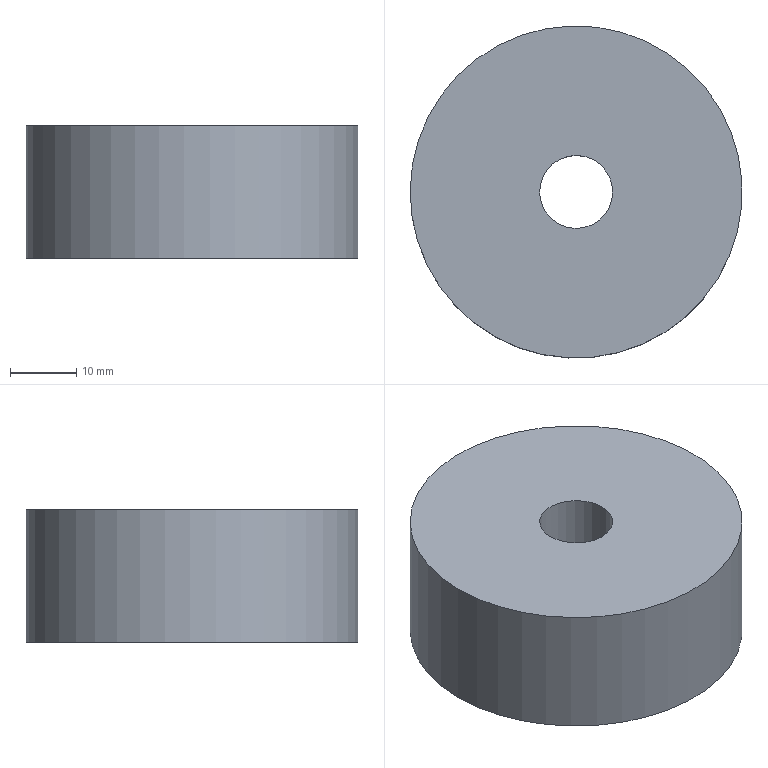Part | NX | features solid 2 | 1 solid | 6 faces | box 50 x 50 x 20 mm | volume 35918 mm3 | cylinder 3 | plane 3 | commonest cylinder face diameters 11 x1 17 x1 50 x1
STEP:
#1=CARTESIAN_POINT('',(-571.907,500.424,300.));
#2=VERTEX_POINT('',#1);
#3=CARTESIAN_POINT('',(-595.,510.,300.));
#4=DIRECTION('',(0.,0.,1.));
#5=DIRECTION('',(0.9237,-0.383,0.));
#6=AXIS2_PLACEMENT_3D('',#3,#4,#5);
#7=CIRCLE('',#6,25.);
#8=EDGE_CURVE('',#2,#2,#7,.T.);
#9=ORIENTED_EDGE('',*,*,#8,.T.);
#10=EDGE_LOOP('',(#9));
#11=FACE_BOUND('',#10,.T.);
#12=CARTESIAN_POINT('',(-571.907,500.424,320.));
#13=VERTEX_POINT('',#12);
#14=CARTESIAN_POINT('',(-595.,510.,320.));
#15=DIRECTION('',(0.,0.,1.));
#16=DIRECTION('',(0.9237,-0.383,0.));
#17=AXIS2_PLACEMENT_3D('',#14,#15,#16);
#18=CIRCLE('',#17,25.);
#19=EDGE_CURVE('',#13,#13,#18,.T.);
#20=ORIENTED_EDGE('',*,*,#19,.F.);
#21=EDGE_LOOP('',(#20));
#22=FACE_BOUND('',#21,.T.);
#23=CARTESIAN_POINT('',(-595.,510.,300.));
#24=DIRECTION('',(0.,0.,1.));
#25=DIRECTION('',(-0.9237,0.383,0.));
#26=AXIS2_PLACEMENT_3D('',#23,#24,#25);
#27=CYLINDRICAL_SURFACE('',#26,25.);
#28=ADVANCED_FACE('',(#11,#22),#27,.T.);
#29=CARTESIAN_POINT('',(-602.852,513.256,300.));
#30=VERTEX_POINT('',#29);
#31=CARTESIAN_POINT('',(-595.,510.,300.));
#32=DIRECTION('',(0.,0.,-1.));
#33=DIRECTION('',(-0.9237,0.383,0.));
#34=AXIS2_PLACEMENT_3D('',#31,#32,#33);
#35=CIRCLE('',#34,8.5);
#36=EDGE_CURVE('',#30,#30,#35,.T.);
#37=ORIENTED_EDGE('',*,*,#36,.F.);
#38=EDGE_LOOP('',(#37));
#39=FACE_BOUND('',#38,.T.);
#40=ORIENTED_EDGE('',*,*,#8,.F.);
#41=EDGE_LOOP('',(#40));
#42=FACE_BOUND('',#41,.T.);
#43=CARTESIAN_POINT('',(-595.,510.,300.));
#44=DIRECTION('',(0.,0.,-1.));
#45=DIRECTION('',(0.9237,-0.383,0.));
#46=AXIS2_PLACEMENT_3D('',#43,#44,#45);
#47=PLANE('',#46);
#48=ADVANCED_FACE('',(#39,#42),#47,.T.);
#49=CARTESIAN_POINT('',(-589.919,507.893,320.));
#50=VERTEX_POINT('',#49);
#51=CARTESIAN_POINT('',(-595.,510.,320.));
#52=DIRECTION('',(0.,0.,1.));
#53=DIRECTION('',(0.9237,-0.383,0.));
#54=AXIS2_PLACEMENT_3D('',#51,#52,#53);
#55=CIRCLE('',#54,5.5);
#56=EDGE_CURVE('',#50,#50,#55,.T.);
#57=ORIENTED_EDGE('',*,*,#56,.F.);
#58=EDGE_LOOP('',(#57));
#59=FACE_BOUND('',#58,.T.);
#60=ORIENTED_EDGE('',*,*,#19,.T.);
#61=EDGE_LOOP('',(#60));
#62=FACE_BOUND('',#61,.T.);
#63=CARTESIAN_POINT('',(-595.,510.,320.));
#64=DIRECTION('',(0.,0.,-1.));
#65=DIRECTION('',(0.9237,-0.383,0.));
#66=AXIS2_PLACEMENT_3D('',#63,#64,#65);
#67=PLANE('',#66);
#68=ADVANCED_FACE('',(#59,#62),#67,.F.);
#69=CARTESIAN_POINT('',(-600.081,512.107,311.));
#70=VERTEX_POINT('',#69);
#71=CARTESIAN_POINT('',(-595.,510.,311.));
#72=DIRECTION('',(0.,0.,-1.));
#73=DIRECTION('',(-0.9237,0.383,0.));
#74=AXIS2_PLACEMENT_3D('',#71,#72,#73);
#75=CIRCLE('',#74,5.5);
#76=EDGE_CURVE('',#70,#70,#75,.T.);
#77=ORIENTED_EDGE('',*,*,#76,.T.);
#78=EDGE_LOOP('',(#77));
#79=FACE_BOUND('',#78,.T.);
#80=ORIENTED_EDGE('',*,*,#56,.T.);
#81=EDGE_LOOP('',(#80));
#82=FACE_BOUND('',#81,.T.);
#83=CARTESIAN_POINT('',(-595.,510.,350.));
#84=DIRECTION('',(0.,0.,1.));
#85=DIRECTION('',(-0.9237,0.383,0.));
#86=AXIS2_PLACEMENT_3D('',#83,#84,#85);
#87=CYLINDRICAL_SURFACE('',#86,5.5);
#88=ADVANCED_FACE('',(#79,#82),#87,.F.);
#89=ORIENTED_EDGE('',*,*,#76,.F.);
#90=EDGE_LOOP('',(#89));
#91=FACE_BOUND('',#90,.T.);
#92=CARTESIAN_POINT('',(-602.852,513.256,311.));
#93=VERTEX_POINT('',#92);
#94=CARTESIAN_POINT('',(-595.,510.,311.));
#95=DIRECTION('',(0.,0.,-1.));
#96=DIRECTION('',(-0.9237,0.383,0.));
#97=AXIS2_PLACEMENT_3D('',#94,#95,#96);
#98=CIRCLE('',#97,8.5);
#99=EDGE_CURVE('',#93,#93,#98,.T.);
#100=ORIENTED_EDGE('',*,*,#99,.T.);
#101=EDGE_LOOP('',(#100));
#102=FACE_BOUND('',#101,.T.);
#103=CARTESIAN_POINT('',(-595.,510.,311.));
#104=DIRECTION('',(0.,0.,1.));
#105=DIRECTION('',(-0.9237,0.383,0.));
#106=AXIS2_PLACEMENT_3D('',#103,#104,#105);
#107=PLANE('',#106);
#108=ADVANCED_FACE('',(#91,#102),#107,.F.);
#109=ORIENTED_EDGE('',*,*,#99,.F.);
#110=EDGE_LOOP('',(#109));
#111=FACE_BOUND('',#110,.T.);
#112=ORIENTED_EDGE('',*,*,#36,.T.);
#113=EDGE_LOOP('',(#112));
#114=FACE_BOUND('',#113,.T.);
#115=CARTESIAN_POINT('',(-595.,510.,300.));
#116=DIRECTION('',(0.,0.,1.));
#117=DIRECTION('',(-0.9237,0.383,0.));
#118=AXIS2_PLACEMENT_3D('',#115,#116,#117);
#119=CYLINDRICAL_SURFACE('',#118,8.5);
#120=ADVANCED_FACE('',(#111,#114),#119,.F.);
#121=CLOSED_SHELL('',(#28,#48,#68,#88,#108,#120));
#122=MANIFOLD_SOLID_BREP('',#121);
#123=(LENGTH_UNIT()NAMED_UNIT(*)SI_UNIT(.MILLI.,.METRE.));
#124=UNCERTAINTY_MEASURE_WITH_UNIT(LENGTH_MEASURE(0.00001),#123,'','');
#125=(NAMED_UNIT(*)PLANE_ANGLE_UNIT()SI_UNIT($,.RADIAN.));
#126=(NAMED_UNIT(*)SI_UNIT($,.STERADIAN.)SOLID_ANGLE_UNIT());
#127=(GEOMETRIC_REPRESENTATION_CONTEXT(3)GLOBAL_UNCERTAINTY_ASSIGNED_CONTEXT((#124))GLOBAL_UNIT_ASSIGNED_CONTEXT((#123,#125,#126))REPRESENTATION_CONTEXT('',''));
#128=ADVANCED_BREP_SHAPE_REPRESENTATION('',(#122),#127);